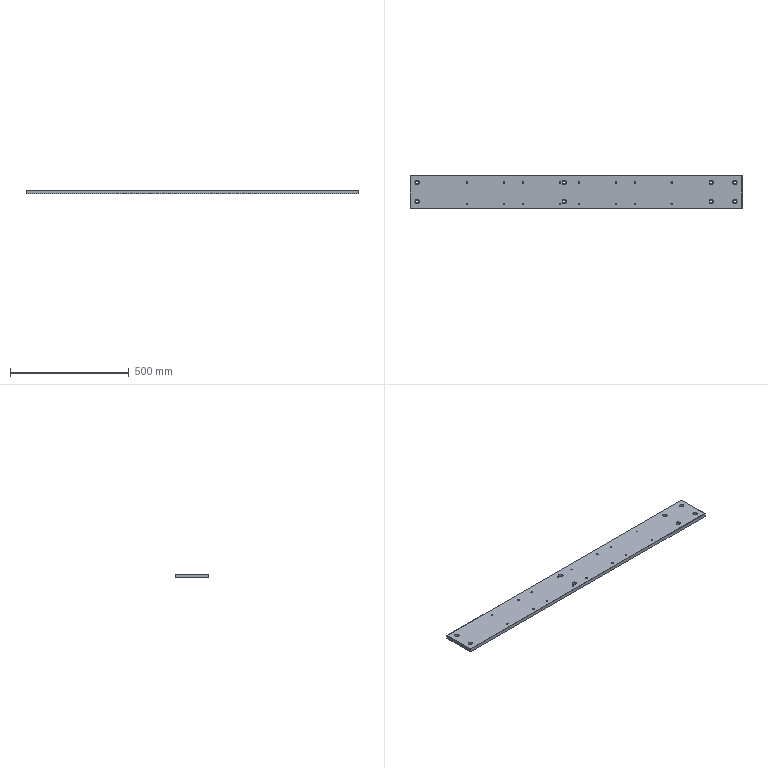Part | SolidWorks | features HoleWzd 3, 3DProfileFeature 2, Chamfer 1, Extrusion 1, LPattern 1 | 1 solid | 82 faces | box 1400 x 140 x 15 mm | volume 2905465 mm3 | cylinder 64 | plane 18 | commonest cylinder face diameters 6.8 x32 11 x16 18 x16